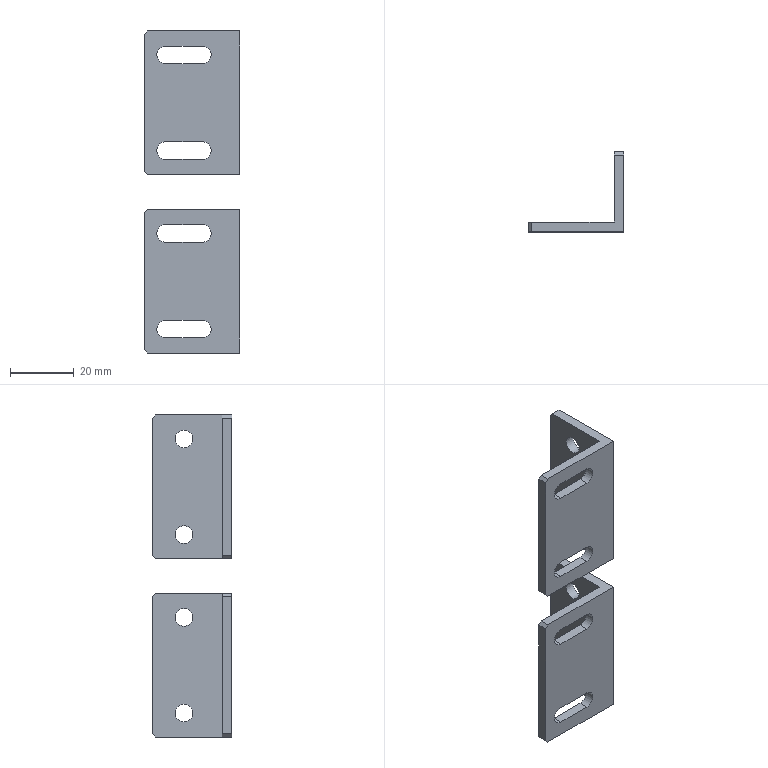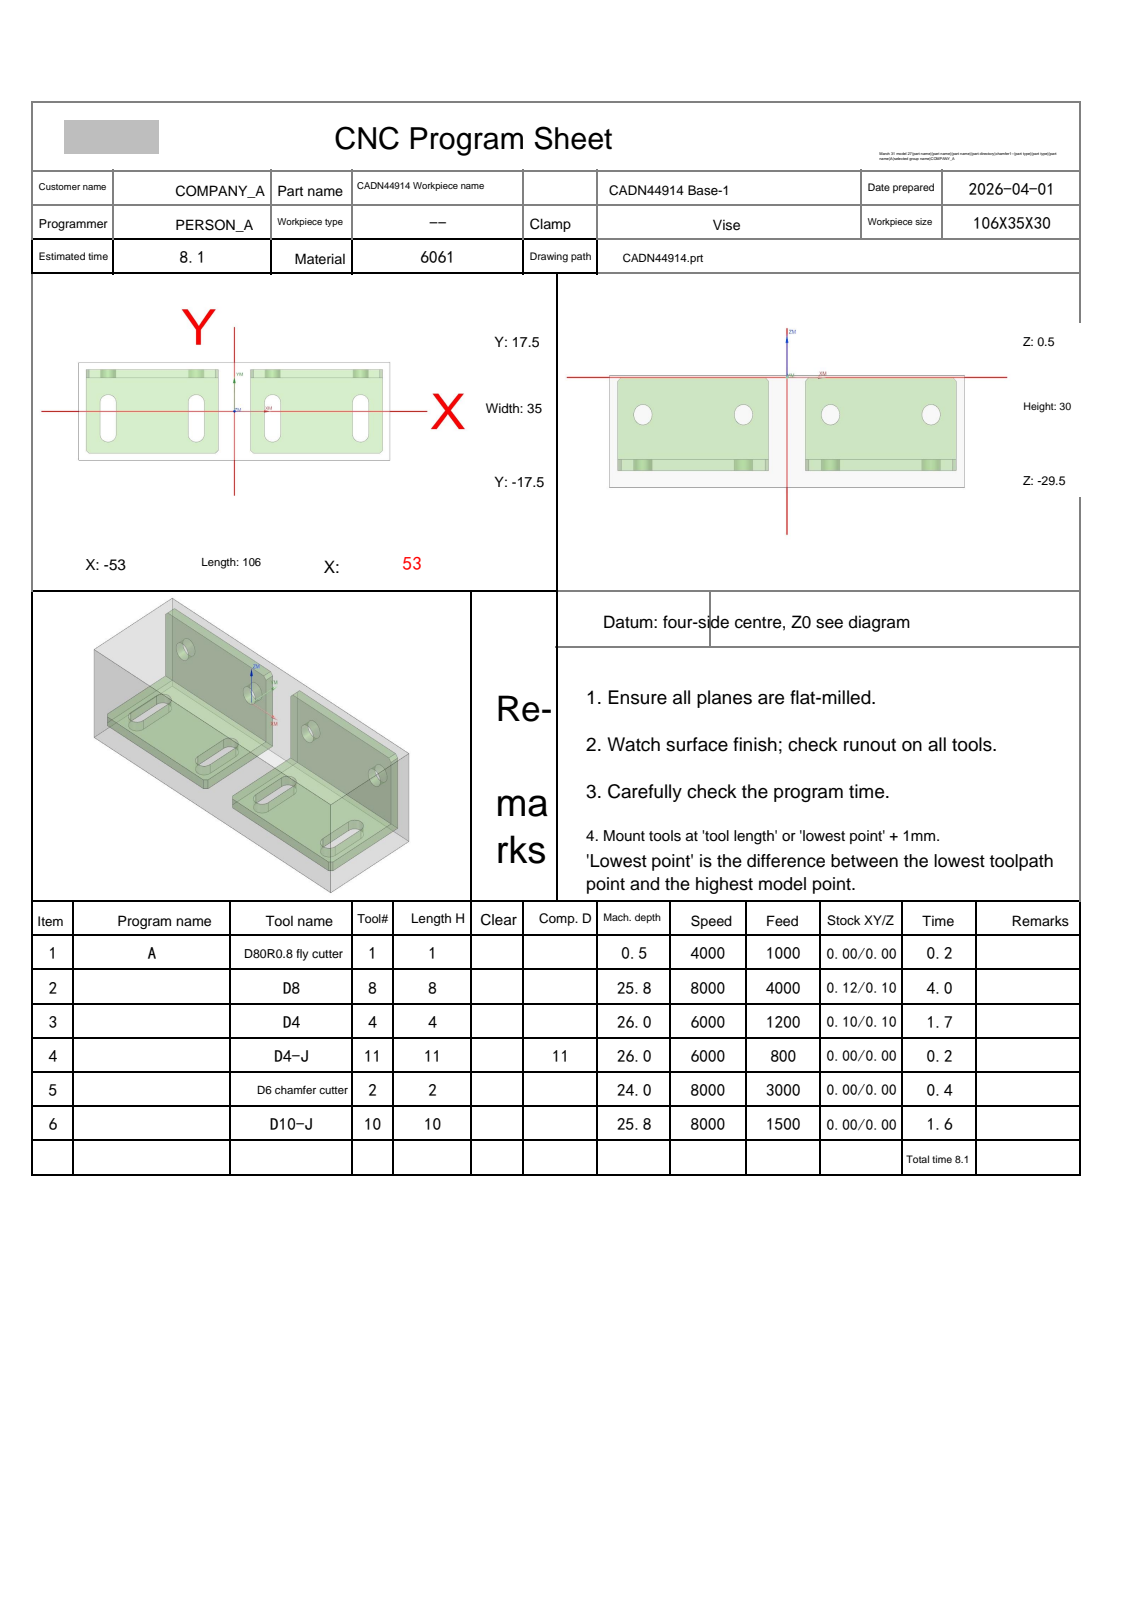NC program | NX | posted by the shop | part box 30 x 25 x 101 mm
Lines 4932 to 5910 of 5910:
N3 T04 M06
(D4  D=4. R=0. H=04 ce=0.10 di=0.10)
G00 G90 G54 X-43.65 Y-2.5 M03 S6000
G43 H04 Z20.
M08
Z-21.5
G01 Y-8.25 Z-21.55 F1200.
G03 X-43. Y-8.9 Z-21.559 I.65 J0.0
X-42.35 Y-8.25 Z-21.568 I0.0 J.65
G01 Y3.25 Z-21.668
G03 X-43. Y3.9 Z-21.676 I-.65 J0.0
X-43.65 Y3.25 Z-21.685 I0.0 J-.65
G01 Y-8.25 Z-21.785
G03 X-43. Y-8.9 Z-21.794 I.65 J0.0
X-42.35 Y-8.25 Z-21.803 I0.0 J.65
G01 Y3.25 Z-21.903
G03 X-43. Y3.9 Z-21.912 I-.65 J0.0
X-43.65 Y3.25 Z-21.921 I0.0 J-.65
G01 Y-8.25 Z-22.021
G03 X-43. Y-8.9 Z-22.029 I.65 J0.0
X-42.35 Y-8.25 Z-22.038 I0.0 J.65
G01 Y3.25 Z-22.138
G03 X-43. Y3.9 Z-22.147 I-.65 J0.0
X-43.65 Y3.25 Z-22.156 I0.0 J-.65
G01 Y-8.25 Z-22.256
G03 X-43. Y-8.9 Z-22.265 I.65 J0.0
X-42.35 Y-8.25 Z-22.274 I0.0 J.65
G01 Y3.25 Z-22.373
G03 X-43. Y3.9 Z-22.382 I-.65 J0.0
X-43.65 Y3.25 Z-22.391 I0.0 J-.65
G01 Y-8.25 Z-22.491
G03 X-43. Y-8.9 Z-22.5 I.65 J0.0
X-42.35 Y-8.25 Z-22.509 I0.0 J.65
G01 Y3.25 Z-22.609
G03 X-43. Y3.9 Z-22.618 I-.65 J0.0
X-43.65 Y3.25 Z-22.627 I0.0 J-.65
G01 Y-8.25 Z-22.726
G03 X-43. Y-8.9 Z-22.735 I.65 J0.0
X-42.35 Y-8.25 Z-22.744 I0.0 J.65
G01 Y3.25 Z-22.844
G03 X-43. Y3.9 Z-22.853 I-.65 J0.0
X-43.65 Y3.25 Z-22.862 I0.0 J-.65
G01 Y-8.25 Z-22.962
G03 X-43. Y-8.9 Z-22.971 I.65 J0.0
X-42.35 Y-8.25 Z-22.979 I0.0 J.65
G01 Y3.25 Z-23.079
G03 X-43. Y3.9 Z-23.088 I-.65 J0.0
X-43.65 Y3.25 Z-23.097 I0.0 J-.65
G01 Y-8.25 Z-23.197
G03 X-43. Y-8.9 Z-23.206 I.65 J0.0
X-42.35 Y-8.25 Z-23.215 I0.0 J.65
G01 Y3.25 Z-23.315
G03 X-43. Y3.9 Z-23.324 I-.65 J0.0
X-43.65 Y3.25 Z-23.332 I0.0 J-.65
G01 Y-8.25 Z-23.432
G03 X-43. Y-8.9 Z-23.441 I.65 J0.0
X-42.35 Y-8.25 Z-23.45 I0.0 J.65
G01 Y3.25 Z-23.55
G03 X-43. Y3.9 Z-23.559 I-.65 J0.0
X-43.65 Y3.25 Z-23.568 I0.0 J-.65
G01 Y-8.25 Z-23.668
G03 X-43. Y-8.9 Z-23.676 I.65 J0.0
X-42.35 Y-8.25 Z-23.685 I0.0 J.65
G01 Y3.25 Z-23.785
G03 X-43. Y3.9 Z-23.794 I-.65 J0.0
X-43.65 Y3.25 Z-23.803 I0.0 J-.65
G01 Y-8.25 Z-23.903
G03 X-43. Y-8.9 Z-23.912 I.65 J0.0
X-42.35 Y-8.25 Z-23.921 I0.0 J.65
G01 Y3.25 Z-24.021
G03 X-43. Y3.9 Z-24.029 I-.65 J0.0
X-43.65 Y3.25 Z-24.038 I0.0 J-.65
G01 Y-8.25 Z-24.138
G03 X-43. Y-8.9 Z-24.147 I.65 J0.0
X-42.35 Y-8.25 Z-24.156 I0.0 J.65
G01 Y3.25 Z-24.256
G03 X-43. Y3.9 Z-24.265 I-.65 J0.0
X-43.65 Y3.25 Z-24.274 I0.0 J-.65
G01 Y-8.25 Z-24.373
G03 X-43. Y-8.9 Z-24.382 I.65 J0.0
X-42.35 Y-8.25 Z-24.391 I0.0 J.65
G01 Y3.25 Z-24.491
G03 X-43. Y3.9 Z-24.5 I-.65 J0.0
X-43.65 Y3.25 Z-24.509 I0.0 J-.65
G01 Y-8.25 Z-24.609
G03 X-43. Y-8.9 Z-24.618 I.65 J0.0
X-42.35 Y-8.25 Z-24.627 I0.0 J.65
G01 Y3.25 Z-24.726
G03 X-43. Y3.9 Z-24.735 I-.65 J0.0
X-43.65 Y3.25 Z-24.744 I0.0 J-.65
G01 Y-8.25 Z-24.844
G03 X-43. Y-8.9 Z-24.853 I.65 J0.0
X-42.35 Y-8.25 Z-24.862 I0.0 J.65
G01 Y3.25 Z-24.962
G03 X-43. Y3.9 Z-24.971 I-.65 J0.0
X-43.65 Y3.25 Z-24.979 I0.0 J-.65
G01 Y-8.25 Z-25.079
G03 X-43. Y-8.9 Z-25.088 I.65 J0.0
X-42.35 Y-8.25 Z-25.097 I0.0 J.65
G01 Y3.25 Z-25.197
G03 X-43. Y3.9 Z-25.206 I-.65 J0.0
X-43.65 Y3.25 Z-25.215 I0.0 J-.65
G01 Y-8.25 Z-25.315
G03 X-43. Y-8.9 Z-25.324 I.65 J0.0
X-42.35 Y-8.25 Z-25.332 I0.0 J.65
G01 Y3.25 Z-25.432
G03 X-43. Y3.9 Z-25.441 I-.65 J0.0
X-43.65 Y3.25 Z-25.45 I0.0 J-.65
G01 Y-2.5 Z-25.5
Y-8.25
G03 X-43. Y-8.9 I.65 J0.0
X-42.35 Y-8.25 I0.0 J.65
G01 Y3.25
G03 X-43. Y3.9 I-.65 J0.0
X-43.65 Y3.25 I0.0 J-.65
G01 Y-2.5
Y-3.
Z-24.5
G00 Z20.
X-13.65 Y-2.5
Z-21.5
G01 Y-8.25 Z-21.55
G03 X-13. Y-8.9 Z-21.559 I.65 J0.0
X-12.35 Y-8.25 Z-21.568 I0.0 J.65
G01 Y3.25 Z-21.668
G03 X-12.444 Y3.587 Z-21.671 I-.65 J0.0
X-13. Y3.9 Z-21.676 I-.556 J-.337
X-13.65 Y3.25 Z-21.685 I0.0 J-.65
G01 Y-8.25 Z-21.785
G03 X-13. Y-8.9 Z-21.794 I.65 J0.0
X-12.35 Y-8.25 Z-21.803 I0.0 J.65
G01 Y3.25 Z-21.903
G03 X-12.444 Y3.587 Z-21.906 I-.65 J0.0
X-13. Y3.9 Z-21.912 I-.556 J-.337
X-13.65 Y3.25 Z-21.921 I0.0 J-.65
G01 Y-8.25 Z-22.021
G03 X-13. Y-8.9 Z-22.029 I.65 J0.0
X-12.35 Y-8.25 Z-22.038 I0.0 J.65
G01 Y3.25 Z-22.138
G03 X-12.444 Y3.587 Z-22.141 I-.65 J0.0
X-13. Y3.9 Z-22.147 I-.556 J-.337
X-13.65 Y3.25 Z-22.156 I0.0 J-.65
G01 Y-8.25 Z-22.256
G03 X-13. Y-8.9 Z-22.265 I.65 J0.0
X-12.35 Y-8.25 Z-22.274 I0.0 J.65
G01 Y3.25 Z-22.373
G03 X-12.444 Y3.587 Z-22.377 I-.65 J0.0
X-13. Y3.9 Z-22.382 I-.556 J-.337
X-13.65 Y3.25 Z-22.391 I0.0 J-.65
G01 Y-8.25 Z-22.491
G03 X-13. Y-8.9 Z-22.5 I.65 J0.0
X-12.35 Y-8.25 Z-22.509 I0.0 J.65
G01 Y3.25 Z-22.609
G03 X-12.444 Y3.587 Z-22.612 I-.65 J0.0
X-13. Y3.9 Z-22.618 I-.556 J-.337
X-13.65 Y3.25 Z-22.627 I0.0 J-.65
G01 Y-8.25 Z-22.726
G03 X-13. Y-8.9 Z-22.735 I.65 J0.0
X-12.35 Y-8.25 Z-22.744 I0.0 J.65
G01 Y3.25 Z-22.844
G03 X-12.444 Y3.587 Z-22.847 I-.65 J0.0
X-13. Y3.9 Z-22.853 I-.556 J-.337
X-13.65 Y3.25 Z-22.862 I0.0 J-.65
G01 Y-8.25 Z-22.962
G03 X-13. Y-8.9 Z-22.971 I.65 J0.0
X-12.35 Y-8.25 Z-22.979 I0.0 J.65
G01 Y3.25 Z-23.079
G03 X-12.444 Y3.587 Z-23.082 I-.65 J0.0
X-13. Y3.9 Z-23.088 I-.556 J-.337
X-13.65 Y3.25 Z-23.097 I0.0 J-.65
G01 Y-8.25 Z-23.197
G03 X-13. Y-8.9 Z-23.206 I.65 J0.0
X-12.35 Y-8.25 Z-23.215 I0.0 J.65
G01 Y3.25 Z-23.315
G03 X-12.444 Y3.587 Z-23.318 I-.65 J0.0
X-13. Y3.9 Z-23.324 I-.556 J-.337
X-13.65 Y3.25 Z-23.332 I0.0 J-.65
G01 Y-8.25 Z-23.432
G03 X-13. Y-8.9 Z-23.441 I.65 J0.0
X-12.35 Y-8.25 Z-23.45 I0.0 J.65
G01 Y3.25 Z-23.55
G03 X-12.444 Y3.587 Z-23.553 I-.65 J0.0
X-13. Y3.9 Z-23.559 I-.556 J-.337
X-13.65 Y3.25 Z-23.568 I0.0 J-.65
G01 Y-8.25 Z-23.668
G03 X-13. Y-8.9 Z-23.676 I.65 J0.0
X-12.35 Y-8.25 Z-23.685 I0.0 J.65
G01 Y3.25 Z-23.785
G03 X-12.444 Y3.587 Z-23.788 I-.65 J0.0
X-13. Y3.9 Z-23.794 I-.556 J-.337
X-13.65 Y3.25 Z-23.803 I0.0 J-.65
G01 Y-8.25 Z-23.903
G03 X-13. Y-8.9 Z-23.912 I.65 J0.0
X-12.35 Y-8.25 Z-23.921 I0.0 J.65
G01 Y3.25 Z-24.021
G03 X-12.444 Y3.587 Z-24.024 I-.65 J0.0
X-13. Y3.9 Z-24.029 I-.556 J-.337
X-13.65 Y3.25 Z-24.038 I0.0 J-.65
G01 Y-8.25 Z-24.138
G03 X-13. Y-8.9 Z-24.147 I.65 J0.0
X-12.35 Y-8.25 Z-24.156 I0.0 J.65
G01 Y3.25 Z-24.256
G03 X-12.444 Y3.587 Z-24.259 I-.65 J0.0
X-13. Y3.9 Z-24.265 I-.556 J-.337
X-13.65 Y3.25 Z-24.274 I0.0 J-.65
G01 Y-8.25 Z-24.373
G03 X-13. Y-8.9 Z-24.382 I.65 J0.0
X-12.35 Y-8.25 Z-24.391 I0.0 J.65
G01 Y3.25 Z-24.491
G03 X-12.444 Y3.587 Z-24.494 I-.65 J0.0
X-13. Y3.9 Z-24.5 I-.556 J-.337
X-13.65 Y3.25 Z-24.509 I0.0 J-.65
G01 Y-8.25 Z-24.609
G03 X-13. Y-8.9 Z-24.618 I.65 J0.0
X-12.35 Y-8.25 Z-24.627 I0.0 J.65
G01 Y3.25 Z-24.726
G03 X-12.444 Y3.587 Z-24.729 I-.65 J0.0
X-13. Y3.9 Z-24.735 I-.556 J-.337
X-13.65 Y3.25 Z-24.744 I0.0 J-.65
G01 Y-8.25 Z-24.844
G03 X-13. Y-8.9 Z-24.853 I.65 J0.0
X-12.35 Y-8.25 Z-24.862 I0.0 J.65
G01 Y3.25 Z-24.962
G03 X-12.444 Y3.587 Z-24.965 I-.65 J0.0
X-13. Y3.9 Z-24.971 I-.556 J-.337
X-13.65 Y3.25 Z-24.979 I0.0 J-.65
G01 Y-8.25 Z-25.079
G03 X-13. Y-8.9 Z-25.088 I.65 J0.0
X-12.35 Y-8.25 Z-25.097 I0.0 J.65
G01 Y3.25 Z-25.197
G03 X-12.444 Y3.587 Z-25.2 I-.65 J0.0
X-13. Y3.9 Z-25.206 I-.556 J-.337
X-13.65 Y3.25 Z-25.215 I0.0 J-.65
G01 Y-8.25 Z-25.315
G03 X-13. Y-8.9 Z-25.324 I.65 J0.0
X-12.35 Y-8.25 Z-25.332 I0.0 J.65
G01 Y3.25 Z-25.432
G03 X-12.444 Y3.587 Z-25.435 I-.65 J0.0
X-13. Y3.9 Z-25.441 I-.556 J-.337
X-13.65 Y3.25 Z-25.45 I0.0 J-.65
G01 Y-2.5 Z-25.5
Y-8.25
G03 X-13. Y-8.9 I.65 J0.0
X-12.35 Y-8.25 I0.0 J.65
G01 Y3.25
G03 X-13. Y3.9 I-.65 J0.0
X-13.65 Y3.25 I0.0 J-.65
G01 Y-2.5
Y-3.
Z-24.5
G00 Z20.
X12.35 Y-2.5
Z-21.5
G01 Y-8.25 Z-21.55
G03 X13. Y-8.9 Z-21.559 I.65 J0.0
X13.65 Y-8.25 Z-21.568 I0.0 J.65
G01 Y3.25 Z-21.668
G03 X13. Y3.9 Z-21.676 I-.65 J0.0
X12.35 Y3.25 Z-21.685 I0.0 J-.65
G01 Y-8.25 Z-21.785
G03 X13. Y-8.9 Z-21.794 I.65 J0.0
X13.65 Y-8.25 Z-21.803 I0.0 J.65
G01 Y3.25 Z-21.903
G03 X13. Y3.9 Z-21.912 I-.65 J0.0
X12.35 Y3.25 Z-21.921 I0.0 J-.65
G01 Y-8.25 Z-22.021
G03 X13. Y-8.9 Z-22.029 I.65 J0.0
X13.65 Y-8.25 Z-22.038 I0.0 J.65
G01 Y3.25 Z-22.138
G03 X13. Y3.9 Z-22.147 I-.65 J0.0
X12.35 Y3.25 Z-22.156 I0.0 J-.65
G01 Y-8.25 Z-22.256
G03 X13. Y-8.9 Z-22.265 I.65 J0.0
X13.65 Y-8.25 Z-22.274 I0.0 J.65
G01 Y3.25 Z-22.373
G03 X13. Y3.9 Z-22.382 I-.65 J0.0
X12.35 Y3.25 Z-22.391 I0.0 J-.65
G01 Y-8.25 Z-22.491
G03 X13. Y-8.9 Z-22.5 I.65 J0.0
X13.65 Y-8.25 Z-22.509 I0.0 J.65
G01 Y3.25 Z-22.609
G03 X13. Y3.9 Z-22.618 I-.65 J0.0
X12.35 Y3.25 Z-22.627 I0.0 J-.65
G01 Y-8.25 Z-22.726
G03 X13. Y-8.9 Z-22.735 I.65 J0.0
X13.65 Y-8.25 Z-22.744 I0.0 J.65
G01 Y3.25 Z-22.844
G03 X13. Y3.9 Z-22.853 I-.65 J0.0
X12.35 Y3.25 Z-22.862 I0.0 J-.65
G01 Y-8.25 Z-22.962
G03 X13. Y-8.9 Z-22.971 I.65 J0.0
X13.65 Y-8.25 Z-22.979 I0.0 J.65
G01 Y3.25 Z-23.079
G03 X13. Y3.9 Z-23.088 I-.65 J0.0
X12.35 Y3.25 Z-23.097 I0.0 J-.65
G01 Y-8.25 Z-23.197
G03 X13. Y-8.9 Z-23.206 I.65 J0.0
X13.65 Y-8.25 Z-23.215 I0.0 J.65
G01 Y3.25 Z-23.315
G03 X13. Y3.9 Z-23.324 I-.65 J0.0
X12.35 Y3.25 Z-23.332 I0.0 J-.65
G01 Y-8.25 Z-23.432
G03 X13. Y-8.9 Z-23.441 I.65 J0.0
X13.65 Y-8.25 Z-23.45 I0.0 J.65
G01 Y3.25 Z-23.55
G03 X13. Y3.9 Z-23.559 I-.65 J0.0
X12.35 Y3.25 Z-23.568 I0.0 J-.65
G01 Y-8.25 Z-23.668
G03 X13. Y-8.9 Z-23.676 I.65 J0.0
X13.65 Y-8.25 Z-23.685 I0.0 J.65
G01 Y3.25 Z-23.785
G03 X13. Y3.9 Z-23.794 I-.65 J0.0
X12.35 Y3.25 Z-23.803 I0.0 J-.65
G01 Y-8.25 Z-23.903
G03 X13. Y-8.9 Z-23.912 I.65 J0.0
X13.65 Y-8.25 Z-23.921 I0.0 J.65
G01 Y3.25 Z-24.021
G03 X13. Y3.9 Z-24.029 I-.65 J0.0
X12.35 Y3.25 Z-24.038 I0.0 J-.65
G01 Y-8.25 Z-24.138
G03 X13. Y-8.9 Z-24.147 I.65 J0.0
X13.65 Y-8.25 Z-24.156 I0.0 J.65
G01 Y3.25 Z-24.256
G03 X13. Y3.9 Z-24.265 I-.65 J0.0
X12.35 Y3.25 Z-24.274 I0.0 J-.65
G01 Y-8.25 Z-24.373
G03 X13. Y-8.9 Z-24.382 I.65 J0.0
X13.65 Y-8.25 Z-24.391 I0.0 J.65
G01 Y3.25 Z-24.491
G03 X13. Y3.9 Z-24.5 I-.65 J0.0
X12.35 Y3.25 Z-24.509 I0.0 J-.65
G01 Y-8.25 Z-24.609
G03 X13. Y-8.9 Z-24.618 I.65 J0.0
X13.65 Y-8.25 Z-24.627 I0.0 J.65
G01 Y3.25 Z-24.726
G03 X13. Y3.9 Z-24.735 I-.65 J0.0
X12.35 Y3.25 Z-24.744 I0.0 J-.65
G01 Y-8.25 Z-24.844
G03 X13. Y-8.9 Z-24.853 I.65 J0.0
X13.65 Y-8.25 Z-24.862 I0.0 J.65
G01 Y3.25 Z-24.962
G03 X13. Y3.9 Z-24.971 I-.65 J0.0
X12.35 Y3.25 Z-24.979 I0.0 J-.65
G01 Y-8.25 Z-25.079
G03 X13. Y-8.9 Z-25.088 I.65 J0.0
X13.65 Y-8.25 Z-25.097 I0.0 J.65
G01 Y3.25 Z-25.197
G03 X13. Y3.9 Z-25.206 I-.65 J0.0
X12.35 Y3.25 Z-25.215 I0.0 J-.65
G01 Y-8.25 Z-25.315
G03 X13. Y-8.9 Z-25.324 I.65 J0.0
X13.65 Y-8.25 Z-25.332 I0.0 J.65
G01 Y3.25 Z-25.432
G03 X13. Y3.9 Z-25.441 I-.65 J0.0
X12.35 Y3.25 Z-25.45 I0.0 J-.65
G01 Y-2.5 Z-25.5
Y-8.25
G03 X13. Y-8.9 I.65 J0.0
X13.65 Y-8.25 I0.0 J.65
G01 Y3.25
G03 X13. Y3.9 I-.65 J0.0
X12.35 Y3.25 I0.0 J-.65
G01 Y-2.5
Y-3.
Z-24.5
G00 Z20.
X43.65 Y-2.5
Z-21.5
G01 Y3.25 Z-21.55
G03 X43. Y3.9 Z-21.559 I-.65 J0.0
X42.35 Y3.25 Z-21.568 I0.0 J-.65
G01 Y-8.25 Z-21.668
G03 X43. Y-8.9 Z-21.676 I.65 J0.0
X43.65 Y-8.25 Z-21.685 I0.0 J.65
G01 Y3.25 Z-21.785
G03 X43. Y3.9 Z-21.794 I-.65 J0.0
X42.35 Y3.25 Z-21.803 I0.0 J-.65
G01 Y-8.25 Z-21.903
G03 X43. Y-8.9 Z-21.912 I.65 J0.0
X43.65 Y-8.25 Z-21.921 I0.0 J.65
G01 Y3.25 Z-22.021
G03 X43. Y3.9 Z-22.029 I-.65 J0.0
X42.35 Y3.25 Z-22.038 I0.0 J-.65
G01 Y-8.25 Z-22.138
G03 X43. Y-8.9 Z-22.147 I.65 J0.0
X43.65 Y-8.25 Z-22.156 I0.0 J.65
G01 Y3.25 Z-22.256
G03 X43. Y3.9 Z-22.265 I-.65 J0.0
X42.35 Y3.25 Z-22.274 I0.0 J-.65
G01 Y-8.25 Z-22.373
G03 X43. Y-8.9 Z-22.382 I.65 J0.0
X43.65 Y-8.25 Z-22.391 I0.0 J.65
G01 Y3.25 Z-22.491
G03 X43. Y3.9 Z-22.5 I-.65 J0.0
X42.35 Y3.25 Z-22.509 I0.0 J-.65
G01 Y-8.25 Z-22.609
G03 X43. Y-8.9 Z-22.618 I.65 J0.0
X43.65 Y-8.25 Z-22.627 I0.0 J.65
G01 Y3.25 Z-22.726
G03 X43. Y3.9 Z-22.735 I-.65 J0.0
X42.35 Y3.25 Z-22.744 I0.0 J-.65
G01 Y-8.25 Z-22.844
G03 X43. Y-8.9 Z-22.853 I.65 J0.0
X43.65 Y-8.25 Z-22.862 I0.0 J.65
G01 Y3.25 Z-22.962
G03 X43. Y3.9 Z-22.971 I-.65 J0.0
X42.35 Y3.25 Z-22.979 I0.0 J-.65
G01 Y-8.25 Z-23.079
G03 X43. Y-8.9 Z-23.088 I.65 J0.0
X43.65 Y-8.25 Z-23.097 I0.0 J.65
G01 Y3.25 Z-23.197
G03 X43. Y3.9 Z-23.206 I-.65 J0.0
X42.35 Y3.25 Z-23.215 I0.0 J-.65
G01 Y-8.25 Z-23.315
G03 X43. Y-8.9 Z-23.324 I.65 J0.0
X43.65 Y-8.25 Z-23.332 I0.0 J.65
G01 Y3.25 Z-23.432
G03 X43. Y3.9 Z-23.441 I-.65 J0.0
X42.35 Y3.25 Z-23.45 I0.0 J-.65
G01 Y-8.25 Z-23.55
G03 X43. Y-8.9 Z-23.559 I.65 J0.0
X43.65 Y-8.25 Z-23.568 I0.0 J.65
G01 Y3.25 Z-23.668
G03 X43. Y3.9 Z-23.676 I-.65 J0.0
X42.35 Y3.25 Z-23.685 I0.0 J-.65
G01 Y-8.25 Z-23.785
G03 X43. Y-8.9 Z-23.794 I.65 J0.0
X43.65 Y-8.25 Z-23.803 I0.0 J.65
G01 Y3.25 Z-23.903
G03 X43. Y3.9 Z-23.912 I-.65 J0.0
X42.35 Y3.25 Z-23.921 I0.0 J-.65
G01 Y-8.25 Z-24.021
G03 X43. Y-8.9 Z-24.029 I.65 J0.0
X43.65 Y-8.25 Z-24.038 I0.0 J.65
G01 Y3.25 Z-24.138
G03 X43. Y3.9 Z-24.147 I-.65 J0.0
X42.35 Y3.25 Z-24.156 I0.0 J-.65
G01 Y-8.25 Z-24.256
G03 X43. Y-8.9 Z-24.265 I.65 J0.0
X43.65 Y-8.25 Z-24.274 I0.0 J.65
G01 Y3.25 Z-24.373
G03 X43. Y3.9 Z-24.382 I-.65 J0.0
X42.35 Y3.25 Z-24.391 I0.0 J-.65
G01 Y-8.25 Z-24.491
G03 X43. Y-8.9 Z-24.5 I.65 J0.0
X43.65 Y-8.25 Z-24.509 I0.0 J.65
G01 Y3.25 Z-24.609
G03 X43. Y3.9 Z-24.618 I-.65 J0.0
X42.35 Y3.25 Z-24.627 I0.0 J-.65
G01 Y-8.25 Z-24.726
G03 X43. Y-8.9 Z-24.735 I.65 J0.0
X43.65 Y-8.25 Z-24.744 I0.0 J.65
G01 Y3.25 Z-24.844
G03 X43. Y3.9 Z-24.853 I-.65 J0.0
X42.35 Y3.25 Z-24.862 I0.0 J-.65
G01 Y-8.25 Z-24.962
G03 X43. Y-8.9 Z-24.971 I.65 J0.0
X43.65 Y-8.25 Z-24.979 I0.0 J.65
G01 Y3.25 Z-25.079
G03 X43. Y3.9 Z-25.088 I-.65 J0.0
X42.35 Y3.25 Z-25.097 I0.0 J-.65
G01 Y-8.25 Z-25.197
G03 X43. Y-8.9 Z-25.206 I.65 J0.0
X43.65 Y-8.25 Z-25.215 I0.0 J.65
G01 Y3.25 Z-25.315
G03 X43. Y3.9 Z-25.324 I-.65 J0.0
X42.35 Y3.25 Z-25.332 I0.0 J-.65
G01 Y-8.25 Z-25.432
G03 X43. Y-8.9 Z-25.441 I.65 J0.0
X43.65 Y-8.25 Z-25.45 I0.0 J.65
G01 Y-2.5 Z-25.5
Y3.25
G03 X43. Y3.9 I-.65 J0.0
X42.35 Y3.25 I0.0 J-.65
G01 Y-8.25
G03 X43. Y-8.9 I.65 J0.0
X43.65 Y-8.25 I0.0 J.65
G01 Y-2.5
Y-2.
Z-24.5
G00 Z20.
G91 G28 Z0.0
M05
M09
G91 G28 Z0.0
M01
N4 T11 M06
(D4-J  D=4. R=0. H=11 ce=0.00 di=0.00)
G00 G90 G54 X-43.5 Y-2.3 M03 S6000
G43 H11 Z20.
M08
Z-25.
G01 Z-25.5 F800.
G41 D11
X-43.55
G03 X-43.75 Y-2.5 I0.0 J-.2
G01 Y-8.25
G03 X-43. Y-9. I.75 J0.0
X-42.25 Y-8.25 I0.0 J.75
G01 Y3.25
G03 X-43. Y4. I-.75 J0.0
X-43.75 Y3.25 I0.0 J-.75
G01 Y-2.5
Y-3.
G03 X-43.55 Y-3.2 I.2 J0.0
G01 G40 X-43.5
Z-25.
G00 Z20.
X-13.5 Y-2.3
Z-25.
G01 Z-25.5
G41 D11
X-13.55
G03 X-13.75 Y-2.5 I0.0 J-.2
G01 Y-8.25
G03 X-13. Y-9. I.75 J0.0
X-12.25 Y-8.25 I0.0 J.75
G01 Y3.25
G03 X-13. Y4. I-.75 J0.0
X-13.75 Y3.25 I0.0 J-.75
G01 Y-2.5
Y-3.
G03 X-13.55 Y-3.2 I.2 J0.0
G01 G40 X-13.5
Z-25.
G00 Z20.
X12.5 Y-2.3
Z-25.
G01 Z-25.5
G41 D11
X12.45
G03 X12.25 Y-2.5 I0.0 J-.2
G01 Y-8.25
G03 X13. Y-9. I.75 J0.0
X13.75 Y-8.25 I0.0 J.75
G01 Y3.25
G03 X13. Y4. I-.75 J0.0
X12.25 Y3.25 I0.0 J-.75
G01 Y-2.5
Y-3.
G03 X12.45 Y-3.2 I.2 J0.0
G01 G40 X12.5
Z-25.
G00 Z20.
X43.5 Y-2.7
Z-25.
G01 Z-25.5
G41 D11
X43.55
G03 X43.75 Y-2.5 I0.0 J.2
G01 Y3.25
G03 X43. Y4. I-.75 J0.0
X42.25 Y3.25 I0.0 J-.75
G01 Y-8.25
G03 X43. Y-9. I.75 J0.0
X43.75 Y-8.25 I0.0 J.75
G01 Y-2.5
Y-2.
G03 X43.55 Y-1.8 I-.2 J0.0
G01 G40 X43.5
Z-25.
G00 Z20.
G91 G28 Z0.0
M05
M09
G91 G28 Z0.0
M01
N5 T02 M06
(D6 chamfer cutter  D=6. R=0. H=02 ce=0.00 di=0.00)
G00 G90 G54 X6.039 Y16.207 M03 S8000
G43 H02 Z20.
M08
Z2.935
G01 Z-1.5 F3000.
X6.211 Y16.267
X6.5 Y16.3
X49.5
X49.789 Y16.267
X49.961 Y16.207
Z2.935
G00 Z3.45
Y10.793
Z2.935
G01 Z-1.5
X49.789 Y10.733
X49.5 Y10.7
X28.
X6.5
X6.211 Y10.733
X6.039 Y10.793
Z2.935
G00 Z20.
X-49.961 Y16.207
Z2.935
G01 Z-1.5
X-49.789 Y16.267
X-49.5 Y16.3
X-6.5
X-6.211 Y16.267
X-6.039 Y16.207
Z2.935
G00 Z3.45
Y10.793
Z2.935
G01 Z-1.5
X-6.211 Y10.733
X-6.5 Y10.7
X-28.
X-49.5
X-49.789 Y10.733
X-49.961 Y10.793
Z2.935
G00 Z20.
X-3.455 Y8.949
Z1.63
G01 Z-23.5
G03 X-3.725 Y9.022 I-.27 J-.468
X-4.193 Y8.752 I0.0 J-.54
G01 X-4.2 Y8.725
Y-14.
X-4.225 Y-14.254
X-4.299 Y-14.497
X-4.419 Y-14.722
X-4.581 Y-14.919
X-5.581 Y-15.919
X-5.778 Y-16.081
X-6.003 Y-16.201
X-6.246 Y-16.275
X-6.5 Y-16.3
X-49.5
X-49.754 Y-16.275
X-49.997 Y-16.201
X-50.222 Y-16.081
X-50.419 Y-15.919
X-51.419 Y-14.919
X-51.581 Y-14.722
X-51.701 Y-14.497
X-51.775 Y-14.254
X-51.8 Y-14.
Y8.725
X-51.807 Y8.752
G03 X-52.275 Y9.022 I-.468 J-.27
X-52.545 Y8.949 I0.0 J-.54
G01 Z1.63
G00 Z20.
X-42.378 Y-2.75
Z-19.901
G01 Z-23.5
G03 X-42.078 Y-2.83 I.3 J.52
X-41.558 Y-2.53 I0.0 J.6
G01 X-41.55 Y-2.5
Y3.25
G03 X-43. Y4.7 I-1.45 J0.0
X-44.45 Y3.25 I0.0 J-1.45
G01 Y-8.25
G03 X-43. Y-9.7 I1.45 J0.0
X-41.55 Y-8.25 I0.0 J1.45
G01 Y-2.5
X-41.558 Y-2.47
G03 X-42.078 Y-2.17 I-.52 J-.3
X-42.378 Y-2.25 I0.0 J-.6
G01 Z-19.901
G00 Z20.
X-13.622
Z-19.901
G01 Z-23.5
G03 X-13.922 Y-2.17 I-.3 J-.52
X-14.442 Y-2.47 I0.0 J-.6
G01 X-14.45 Y-2.5
Y-8.25
G03 X-13. Y-9.7 I1.45 J0.0
X-11.55 Y-8.25 I0.0 J1.45
G01 Y3.25
G03 X-13. Y4.7 I-1.45 J0.0
X-14.45 Y3.25 I0.0 J-1.45
G01 Y-2.5
X-14.442 Y-2.53
G03 X-13.922 Y-2.83 I.52 J.3
X-13.622 Y-2.75 I0.0 J.6
G01 Z-19.901
G00 Z20.
X52.545 Y8.949
Z1.63
G01 Z-23.5
G03 X52.275 Y9.022 I-.27 J-.468
X51.807 Y8.752 I0.0 J-.54
G01 X51.8 Y8.725
Y-14.
X51.775 Y-14.254
X51.701 Y-14.497
X51.581 Y-14.722
X51.419 Y-14.919
X50.419 Y-15.919
X50.222 Y-16.081
X49.997 Y-16.201
X49.754 Y-16.275
X49.5 Y-16.3
X6.5
X6.246 Y-16.275
X6.003 Y-16.201
X5.778 Y-16.081
X5.581 Y-15.919
X4.581 Y-14.919
X4.419 Y-14.722
X4.299 Y-14.497
X4.225 Y-14.254
X4.2 Y-14.
Y8.725
X4.193 Y8.752
G03 X3.725 Y9.022 I-.468 J-.27
X3.455 Y8.949 I0.0 J-.54
G01 Z1.63
G00 Z20.
X12.378 Y-2.25
Z-19.901
G01 Z-23.5
G03 X12.078 Y-2.17 I-.3 J-.52
X11.558 Y-2.47 I0.0 J-.6
G01 X11.55 Y-2.5
Y-8.25
G03 X13. Y-9.7 I1.45 J0.0
X14.45 Y-8.25 I0.0 J1.45
G01 Y3.25
G03 X13. Y4.7 I-1.45 J0.0
X11.55 Y3.25 I0.0 J-1.45
G01 Y-2.5
X11.558 Y-2.53
G03 X12.078 Y-2.83 I.52 J.3
X12.378 Y-2.75 I0.0 J.6
G01 Z-19.901
G00 Z20.
X42.378 Y-2.25
Z-19.901
G01 Z-23.5
G03 X42.078 Y-2.17 I-.3 J-.52
X41.558 Y-2.47 I0.0 J-.6
G01 X41.55 Y-2.5
Y-8.25
G03 X43. Y-9.7 I1.45 J0.0
X44.45 Y-8.25 I0.0 J1.45
G01 Y3.25
G03 X43. Y4.7 I-1.45 J0.0
X41.55 Y3.25 I0.0 J-1.45
G01 Y-2.5
X41.558 Y-2.53
G03 X42.078 Y-2.83 I.52 J.3
X42.378 Y-2.75 I0.0 J.6
G01 Z-19.901
G00 Z20.
G00 G90 X51.208 Y17.9 M03 S6500
Z20.
Z-.2
G01 Z-1.7 F1500.
X51.199 Y17.832
X51.2 Y17.763
Y9.237
X51.199 Y9.168
X51.208 Y9.1
Z-.2
G00 Z20.
X-4.792 Y17.9
Z-.2
G01 Z-1.7
X-4.801 Y17.832
X-4.8 Y17.763
Y9.237
X-4.801 Y9.168
X-4.792 Y9.1
Z-.2
G00 Z20.
X4.792
Z-.2
G01 Z-1.7
X4.801 Y9.168
X4.8 Y9.237
Y17.763
X4.801 Y17.832
X4.792 Y17.9
Z-.2
G00 Z20.
X-51.208 Y9.1
Z-.2
G01 Z-1.7
X-51.199 Y9.168
X-51.2 Y9.237
Y17.763
X-51.199 Y17.832
X-51.208 Y17.9
Z-.2
G00 Z20.
G91 G28 Z0.0
M05
M09
G91 G28 Z0.0
M01
N6 T10 M06
(D10-J  D=10. R=0. H=10 ce=0.40 di=0.00)
G00 G90 G54 X57.252 Y-17.036 M03 S7000
G43 H10 Z10.5
M08
Z-20.5
G01 Z-22. F1500.
G03 X55.5 Y-16. I-1.752 J-.964
G01 X-54.6
G02 X-55.5 Y-15.1 I0.0 J.9
G01 Y-12.48
G02 X-54.5 Y-11.48 I1. J0.0
G01 X54.6
G03 X55.5 Y-10.58 I0.0 J.9
G01 Y-7.96
G03 X54.5 Y-6.96 I-1. J0.0
G01 X-54.6
G02 X-55.5 Y-6.06 I0.0 J.9
G01 Y-3.44
G02 X-54.5 Y-2.44 I1. J0.0
G01 X54.6
G03 X55.5 Y-1.54 I0.0 J.9
G01 Y1.08
G03 X54.5 Y2.08 I-1. J0.0
G01 X-54.6
G02 X-55.5 Y2.98 I0.0 J.9
G01 Y5.6
G02 X-54.5 Y6.6 I1. J0.0
G01 X55.5
G02 X57.5 Y4.6 I0.0 J-2.
G01 Z-20.5
G00 Z10.5
G00 G90 X3.987 Y21.526 M03 S8000
Z5.5
Z-7.433
G01 Z-8.433 F1000.
G41 D10
X4.01 Y21.327
G03 X5.5 Y20. I1.49 J.173
G01 X50.5
G02 X55.5 Y15. I0.0 J-5.
G01 Y11.977
G02 X50.5 Y7. I-5. J.023
G01 X5.5
G02 X.5 Y12. I0.0 J5.
G01 Y15.
G02 X5.5 Y20. I5. J0.0
G03 X7. Y21.5 I0.0 J1.5
G01 G40 Y21.7
Z-7.433
G00 Z5.5
X-52.013 Y21.526
Z-7.433
G01 Z-8.433
G41 D10
X-51.99 Y21.327
G03 X-50.5 Y20. I1.49 J.173
G01 X-5.5
G02 X-.5 Y15. I0.0 J-5.
G01 Y12.
G02 X-5.5 Y7. I-5. J0.0
G01 X-50.5
G02 X-55.5 Y12. I0.0 J5.
G01 Y15.
G02 X-50.5 Y20. I5. J0.0
G03 X-49. Y21.5 I0.0 J1.5
G01 G40 Y21.7
Z-7.433
G00 X-52.013 Y21.526
Z-15.867
G01 Z-16.867
G41 D10
X-51.99 Y21.327
G03 X-50.5 Y20. I1.49 J.173
G01 X-5.5
G02 X-.5 Y15. I0.0 J-5.
G01 Y12.
G02 X-5.5 Y7. I-5. J0.0
G01 X-50.5
G02 X-55.5 Y11.967 I0.0 J5.
G01 Y12.
Y15.
G02 X-50.5 Y20. I5. J0.0
G03 X-49. Y21.5 I0.0 J1.5
G01 G40 Y21.7
Z-15.867
G00 Z5.5
X3.987 Y21.526
Z-15.867
G01 Z-16.867
G41 D10
X4.01 Y21.327
G03 X5.5 Y20. I1.49 J.173
G01 X50.5
G02 X55.5 Y15. I0.0 J-5.
G01 Y12.
Y11.967
G02 X50.5 Y7. I-5. J.033
G01 X5.5
G02 X.5 Y12. I0.0 J5.
G01 Y15.
G02 X5.5 Y20. I5. J0.0
G03 X7. Y21.5 I0.0 J1.5
G01 G40 Y21.7
Z-15.867
G00 Z5.5
X57.2 Y13.496
Z-21.
G01 Z-22.
G41 D10
X57.
G03 X55.5 Y12.001 I0.0 J-1.5
G01 Y11.967
G02 X50.5 Y7. I-5. J.033
G01 X5.5
G02 X.5 Y12. I0.0 J5.
G01 Y12.001
G03 X-.25 Y12.751 I-.75 J0.0
G01 G40 X0.0 Y8.536
Z-21.
G00 Z5.5
Z-21.
G01 Z-22.
G41 D10
X.25 Y12.751
G03 X-.5 Y12.001 I0.0 J-.75
G02 X-5.5 Y7. I-5. J0.0
G01 X-50.5
G02 X-55.5 Y11.967 I0.0 J5.
G01 Y12.001
G03 X-57. Y13.496 I-1.5 J-.005
G01 G40 X-57.2
Z-21.
G00 Z5.5
X3.987 Y21.526
Z-24.3
G01 Z-25.3
G41 D10
X4.01 Y21.327
G03 X5.5 Y20. I1.49 J.173
G01 X50.5
G02 X55.5 Y15. I0.0 J-5.
G01 Y-14.
G02 X54.036 Y-17.536 I-5. J0.0
G01 X53.036 Y-18.536
G02 X49.5 Y-20. I-3.536 J3.536
G01 X6.5
G02 X2.964 Y-18.536 I0.0 J5.
G01 X1.964 Y-17.536
G02 X.5 Y-14. I3.536 J3.536
G01 Y15.
G02 X5.5 Y20. I5. J0.0
G03 X7. Y21.5 I0.0 J1.5
G01 G40 Y21.7
Z-24.3
G00 Z5.5
X-52.013 Y21.526
Z-24.3
G01 Z-25.3
G41 D10
X-51.99 Y21.327
G03 X-50.5 Y20. I1.49 J.173
G01 X-5.5
G02 X-.5 Y15. I0.0 J-5.
G01 Y-14.
G02 X-1.964 Y-17.536 I-5. J0.0
G01 X-2.964 Y-18.536
G02 X-6.5 Y-20. I-3.536 J3.536
G01 X-49.5
G02 X-53.036 Y-18.536 I0.0 J5.
G01 X-54.036 Y-17.536
G02 X-55.5 Y-14. I3.536 J3.536
G01 Y15.
G02 X-50.5 Y20. I5. J0.0
G03 X-49. Y21.5 I0.0 J1.5
G01 G40 Y21.7
Z-24.3
G00 Z5.5
M05
M09
G91 G28 Z0.0
G91 G28 Y0.0
M30
%